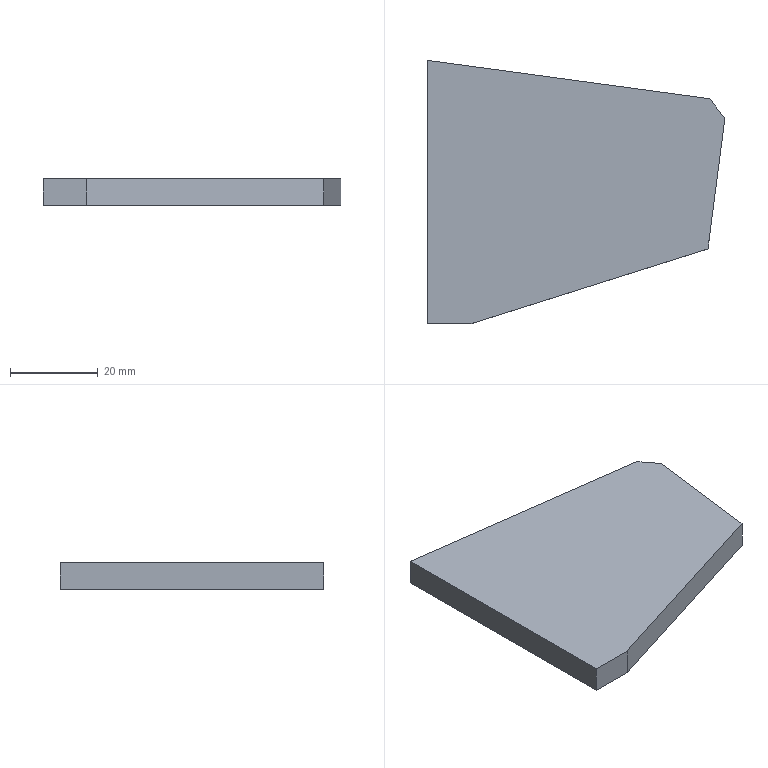Part | SolidWorks | features Chamfer 1, Extrusion 1 | 1 solid | 8 faces | box 67.858 x 60 x 6 mm | volume 19020 mm3 | plane 8
STEP:
#1=CARTESIAN_POINT('',(0.,60.,6.));
#2=VERTEX_POINT('',#1);
#3=CARTESIAN_POINT('',(64.385,51.26,6.));
#4=VERTEX_POINT('',#3);
#5=CARTESIAN_POINT('',(0.,60.,6.));
#6=DIRECTION('',(0.9909,-0.1345,0.));
#7=VECTOR('',#6,1000.);
#8=LINE('',#5,#7);
#9=EDGE_CURVE('',#2,#4,#8,.T.);
#10=ORIENTED_EDGE('',*,*,#9,.T.);
#11=CARTESIAN_POINT('',(64.385,51.26,0.));
#12=VERTEX_POINT('',#11);
#13=CARTESIAN_POINT('',(64.385,51.26,6.));
#14=DIRECTION('',(0.,0.,-1.));
#15=VECTOR('',#14,1000.);
#16=LINE('',#13,#15);
#17=EDGE_CURVE('',#4,#12,#16,.T.);
#18=ORIENTED_EDGE('',*,*,#17,.T.);
#19=CARTESIAN_POINT('',(0.,60.,0.));
#20=VERTEX_POINT('',#19);
#21=CARTESIAN_POINT('',(0.,60.,0.));
#22=DIRECTION('',(0.9909,-0.1345,0.));
#23=VECTOR('',#22,1000.);
#24=LINE('',#21,#23);
#25=EDGE_CURVE('',#20,#12,#24,.T.);
#26=ORIENTED_EDGE('',*,*,#25,.F.);
#27=CARTESIAN_POINT('',(0.,60.,6.));
#28=DIRECTION('',(0.,0.,-1.));
#29=VECTOR('',#28,1000.);
#30=LINE('',#27,#29);
#31=EDGE_CURVE('',#2,#20,#30,.T.);
#32=ORIENTED_EDGE('',*,*,#31,.F.);
#33=EDGE_LOOP('',(#10,#18,#26,#32));
#34=FACE_OUTER_BOUND('',#33,.T.);
#35=CARTESIAN_POINT('',(0.,60.,6.));
#36=DIRECTION('',(0.1345,0.9909,0.));
#37=DIRECTION('',(-0.9909,0.1345,0.));
#38=AXIS2_PLACEMENT_3D('',#35,#36,#37);
#39=PLANE('',#38);
#40=ADVANCED_FACE('',(#34),#39,.T.);
#41=CARTESIAN_POINT('',(0.,0.,0.));
#42=VERTEX_POINT('',#41);
#43=CARTESIAN_POINT('',(0.,0.,0.));
#44=DIRECTION('',(0.,1.,0.));
#45=VECTOR('',#44,1000.);
#46=LINE('',#43,#45);
#47=EDGE_CURVE('',#42,#20,#46,.T.);
#48=ORIENTED_EDGE('',*,*,#47,.F.);
#49=CARTESIAN_POINT('',(0.,0.,6.));
#50=VERTEX_POINT('',#49);
#51=CARTESIAN_POINT('',(0.,0.,6.));
#52=DIRECTION('',(0.,0.,-1.));
#53=VECTOR('',#52,1000.);
#54=LINE('',#51,#53);
#55=EDGE_CURVE('',#50,#42,#54,.T.);
#56=ORIENTED_EDGE('',*,*,#55,.F.);
#57=CARTESIAN_POINT('',(0.,0.,6.));
#58=DIRECTION('',(0.,1.,0.));
#59=VECTOR('',#58,1000.);
#60=LINE('',#57,#59);
#61=EDGE_CURVE('',#50,#2,#60,.T.);
#62=ORIENTED_EDGE('',*,*,#61,.T.);
#63=ORIENTED_EDGE('',*,*,#31,.T.);
#64=EDGE_LOOP('',(#48,#56,#62,#63));
#65=FACE_OUTER_BOUND('',#64,.T.);
#66=CARTESIAN_POINT('',(0.,0.,6.));
#67=DIRECTION('',(-1.,0.,0.));
#68=DIRECTION('',(0.,0.,1.));
#69=AXIS2_PLACEMENT_3D('',#66,#67,#68);
#70=PLANE('',#69);
#71=ADVANCED_FACE('',(#65),#70,.T.);
#72=CARTESIAN_POINT('',(10.,0.,0.));
#73=VERTEX_POINT('',#72);
#74=CARTESIAN_POINT('',(10.,0.,0.));
#75=DIRECTION('',(-1.,0.,0.));
#76=VECTOR('',#75,1000.);
#77=LINE('',#74,#76);
#78=EDGE_CURVE('',#73,#42,#77,.T.);
#79=ORIENTED_EDGE('',*,*,#78,.F.);
#80=CARTESIAN_POINT('',(10.,0.,6.));
#81=VERTEX_POINT('',#80);
#82=CARTESIAN_POINT('',(10.,0.,6.));
#83=DIRECTION('',(0.,0.,-1.));
#84=VECTOR('',#83,1000.);
#85=LINE('',#82,#84);
#86=EDGE_CURVE('',#81,#73,#85,.T.);
#87=ORIENTED_EDGE('',*,*,#86,.F.);
#88=CARTESIAN_POINT('',(10.,0.,6.));
#89=DIRECTION('',(-1.,0.,0.));
#90=VECTOR('',#89,1000.);
#91=LINE('',#88,#90);
#92=EDGE_CURVE('',#81,#50,#91,.T.);
#93=ORIENTED_EDGE('',*,*,#92,.T.);
#94=ORIENTED_EDGE('',*,*,#55,.T.);
#95=EDGE_LOOP('',(#79,#87,#93,#94));
#96=FACE_OUTER_BOUND('',#95,.T.);
#97=CARTESIAN_POINT('',(10.,0.,6.));
#98=DIRECTION('',(0.,-1.,0.));
#99=DIRECTION('',(1.,0.,0.));
#100=AXIS2_PLACEMENT_3D('',#97,#98,#99);
#101=PLANE('',#100);
#102=ADVANCED_FACE('',(#96),#101,.T.);
#103=CARTESIAN_POINT('',(64.,17.,0.));
#104=VERTEX_POINT('',#103);
#105=CARTESIAN_POINT('',(64.,17.,0.));
#106=DIRECTION('',(-0.9538,-0.3003,0.));
#107=VECTOR('',#106,1000.);
#108=LINE('',#105,#107);
#109=EDGE_CURVE('',#104,#73,#108,.T.);
#110=ORIENTED_EDGE('',*,*,#109,.F.);
#111=CARTESIAN_POINT('',(64.,17.,6.));
#112=VERTEX_POINT('',#111);
#113=CARTESIAN_POINT('',(64.,17.,6.));
#114=DIRECTION('',(0.,0.,-1.));
#115=VECTOR('',#114,1000.);
#116=LINE('',#113,#115);
#117=EDGE_CURVE('',#112,#104,#116,.T.);
#118=ORIENTED_EDGE('',*,*,#117,.F.);
#119=CARTESIAN_POINT('',(64.,17.,6.));
#120=DIRECTION('',(-0.9538,-0.3003,0.));
#121=VECTOR('',#120,1000.);
#122=LINE('',#119,#121);
#123=EDGE_CURVE('',#112,#81,#122,.T.);
#124=ORIENTED_EDGE('',*,*,#123,.T.);
#125=ORIENTED_EDGE('',*,*,#86,.T.);
#126=EDGE_LOOP('',(#110,#118,#124,#125));
#127=FACE_OUTER_BOUND('',#126,.T.);
#128=CARTESIAN_POINT('',(64.,17.,6.));
#129=DIRECTION('',(0.3003,-0.9538,0.));
#130=DIRECTION('',(0.9538,0.3003,0.));
#131=AXIS2_PLACEMENT_3D('',#128,#129,#130);
#132=PLANE('',#131);
#133=ADVANCED_FACE('',(#127),#132,.T.);
#134=CARTESIAN_POINT('',(67.858,46.751,0.));
#135=VERTEX_POINT('',#134);
#136=CARTESIAN_POINT('',(68.373,50.718,0.));
#137=DIRECTION('',(-0.1286,-0.9917,0.));
#138=VECTOR('',#137,1000.);
#139=LINE('',#136,#138);
#140=EDGE_CURVE('',#135,#104,#139,.T.);
#141=ORIENTED_EDGE('',*,*,#140,.F.);
#142=CARTESIAN_POINT('',(67.858,46.751,6.));
#143=VERTEX_POINT('',#142);
#144=CARTESIAN_POINT('',(67.858,46.751,6.));
#145=DIRECTION('',(0.,0.,1.));
#146=VECTOR('',#145,1000.);
#147=LINE('',#144,#146);
#148=EDGE_CURVE('',#135,#143,#147,.T.);
#149=ORIENTED_EDGE('',*,*,#148,.T.);
#150=CARTESIAN_POINT('',(68.373,50.718,6.));
#151=DIRECTION('',(-0.1286,-0.9917,0.));
#152=VECTOR('',#151,1000.);
#153=LINE('',#150,#152);
#154=EDGE_CURVE('',#143,#112,#153,.T.);
#155=ORIENTED_EDGE('',*,*,#154,.T.);
#156=ORIENTED_EDGE('',*,*,#117,.T.);
#157=EDGE_LOOP('',(#141,#149,#155,#156));
#158=FACE_OUTER_BOUND('',#157,.T.);
#159=CARTESIAN_POINT('',(68.373,50.718,6.));
#160=DIRECTION('',(0.9917,-0.1286,0.));
#161=DIRECTION('',(0.1286,0.9917,0.));
#162=AXIS2_PLACEMENT_3D('',#159,#160,#161);
#163=PLANE('',#162);
#164=ADVANCED_FACE('',(#158),#163,.T.);
#165=ORIENTED_EDGE('',*,*,#154,.F.);
#166=CARTESIAN_POINT('',(64.385,51.26,6.));
#167=DIRECTION('',(-0.6103,0.7922,0.));
#168=VECTOR('',#167,1000.);
#169=LINE('',#166,#168);
#170=EDGE_CURVE('',#143,#4,#169,.T.);
#171=ORIENTED_EDGE('',*,*,#170,.T.);
#172=ORIENTED_EDGE('',*,*,#9,.F.);
#173=ORIENTED_EDGE('',*,*,#61,.F.);
#174=ORIENTED_EDGE('',*,*,#92,.F.);
#175=ORIENTED_EDGE('',*,*,#123,.F.);
#176=EDGE_LOOP('',(#165,#171,#172,#173,#174,#175));
#177=FACE_OUTER_BOUND('',#176,.T.);
#178=CARTESIAN_POINT('',(0.,0.,6.));
#179=DIRECTION('',(0.,0.,-1.));
#180=DIRECTION('',(-1.,0.,0.));
#181=AXIS2_PLACEMENT_3D('',#178,#179,#180);
#182=PLANE('',#181);
#183=ADVANCED_FACE('',(#177),#182,.F.);
#184=ORIENTED_EDGE('',*,*,#25,.T.);
#185=CARTESIAN_POINT('',(65.187,50.22,0.));
#186=DIRECTION('',(0.6103,-0.7922,0.));
#187=VECTOR('',#186,1000.);
#188=LINE('',#185,#187);
#189=EDGE_CURVE('',#12,#135,#188,.T.);
#190=ORIENTED_EDGE('',*,*,#189,.T.);
#191=ORIENTED_EDGE('',*,*,#140,.T.);
#192=ORIENTED_EDGE('',*,*,#109,.T.);
#193=ORIENTED_EDGE('',*,*,#78,.T.);
#194=ORIENTED_EDGE('',*,*,#47,.T.);
#195=EDGE_LOOP('',(#184,#190,#191,#192,#193,#194));
#196=FACE_OUTER_BOUND('',#195,.T.);
#197=CARTESIAN_POINT('',(0.,0.,0.));
#198=DIRECTION('',(0.,0.,-1.));
#199=DIRECTION('',(-1.,0.,0.));
#200=AXIS2_PLACEMENT_3D('',#197,#198,#199);
#201=PLANE('',#200);
#202=ADVANCED_FACE('',(#196),#201,.T.);
#203=ORIENTED_EDGE('',*,*,#170,.F.);
#204=ORIENTED_EDGE('',*,*,#148,.F.);
#205=ORIENTED_EDGE('',*,*,#189,.F.);
#206=ORIENTED_EDGE('',*,*,#17,.F.);
#207=EDGE_LOOP('',(#203,#204,#205,#206));
#208=FACE_OUTER_BOUND('',#207,.T.);
#209=CARTESIAN_POINT('',(64.385,51.26,6.));
#210=DIRECTION('',(-0.7922,-0.6103,0.));
#211=DIRECTION('',(0.,0.,-1.));
#212=AXIS2_PLACEMENT_3D('',#209,#210,#211);
#213=PLANE('',#212);
#214=ADVANCED_FACE('',(#208),#213,.F.);
#215=CLOSED_SHELL('',(#40,#71,#102,#133,#164,#183,#202,#214));
#216=MANIFOLD_SOLID_BREP('',#215);
#217=CARTESIAN_POINT('',(0.,0.,0.));
#218=DIRECTION('',(0.,0.,1.));
#219=DIRECTION('',(1.,0.,0.));
#220=AXIS2_PLACEMENT_3D('',#217,#218,#219);
#221=(LENGTH_UNIT()NAMED_UNIT(*)SI_UNIT(.MILLI.,.METRE.));
#222=UNCERTAINTY_MEASURE_WITH_UNIT(LENGTH_MEASURE(0.00001),#221,'','');
#223=(NAMED_UNIT(*)PLANE_ANGLE_UNIT()SI_UNIT($,.RADIAN.));
#224=(NAMED_UNIT(*)SI_UNIT($,.STERADIAN.)SOLID_ANGLE_UNIT());
#225=(GEOMETRIC_REPRESENTATION_CONTEXT(3)GLOBAL_UNCERTAINTY_ASSIGNED_CONTEXT((#222))GLOBAL_UNIT_ASSIGNED_CONTEXT((#221,#223,#224))REPRESENTATION_CONTEXT('',''));
#226=ADVANCED_BREP_SHAPE_REPRESENTATION('',(#216,#220),#225);